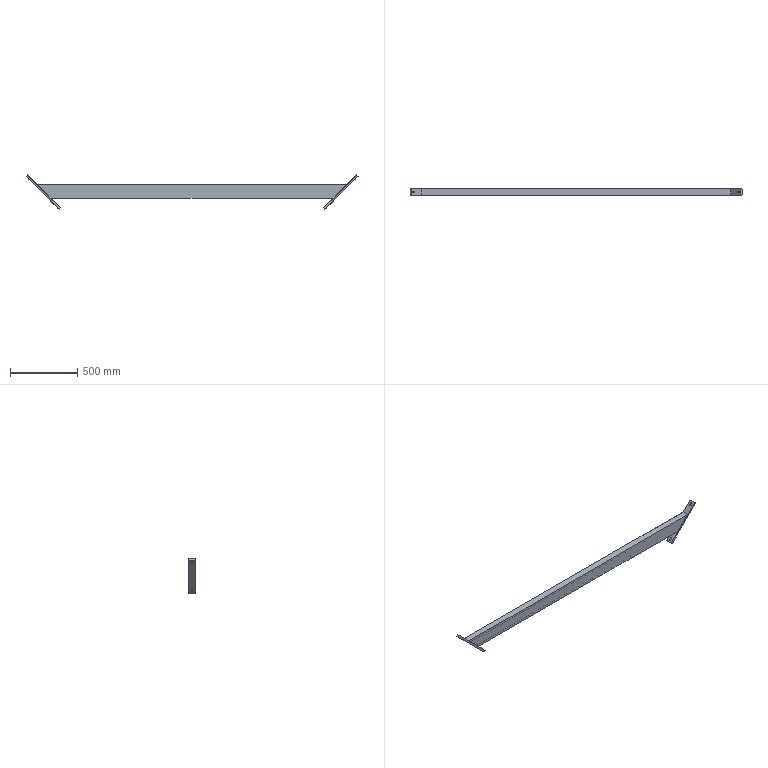Part | SolidWorks | features ICE 2, MirrorSolid 1, WeldMemberFeat 1, WeldmentFeature 1 | 3 solids | 54 faces | box 2475 x 48 x 257.387 mm | volume 3266090 mm3 | plane 30 | cylinder 24 | commonest cylinder face diameters 14 x12 10 x8 8.4 x2 17 x2